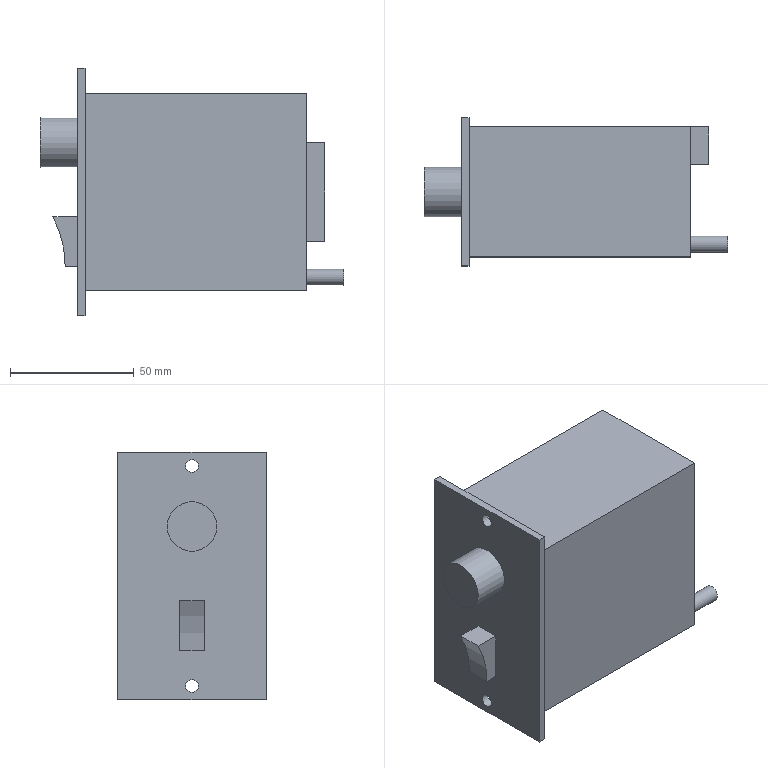Part | STEP file | Speed control panel | 1 solid | 26 faces | box 122.5 x 60 x 100 mm | volume 404808 mm3 | plane 21 | cylinder 5 | commonest cylinder face diameters 5.2 x2 6.5 x1 20 x1 85 x1